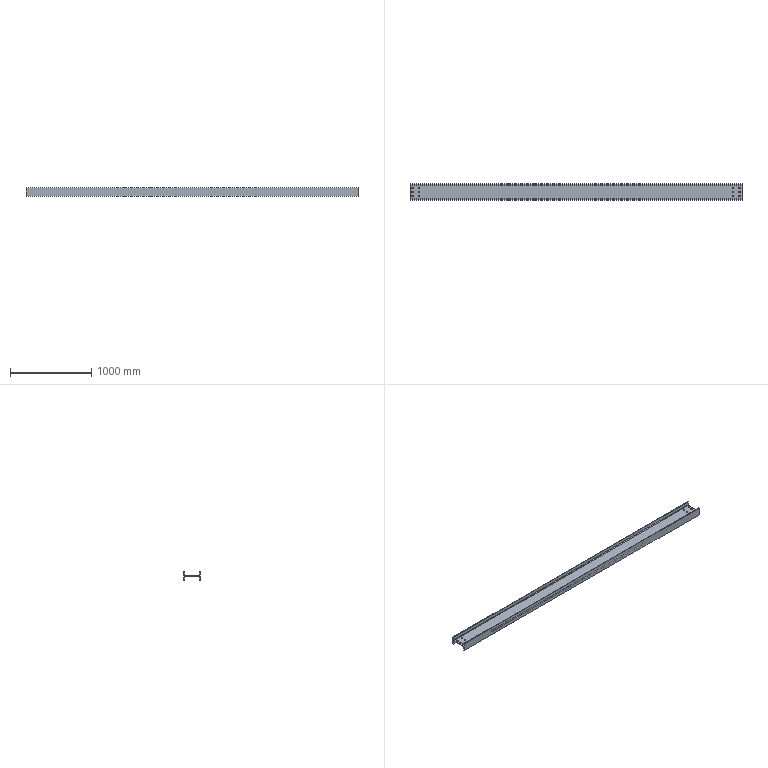Part | STEP file | Electrical cabinet main beam 6 body_Default<As Machined> | 1 solid | 42 faces | box 4080 x 200 x 100 mm | volume 10862394 mm3 | cylinder 28 | plane 14 | commonest cylinder face diameters 19 x24 16 x4